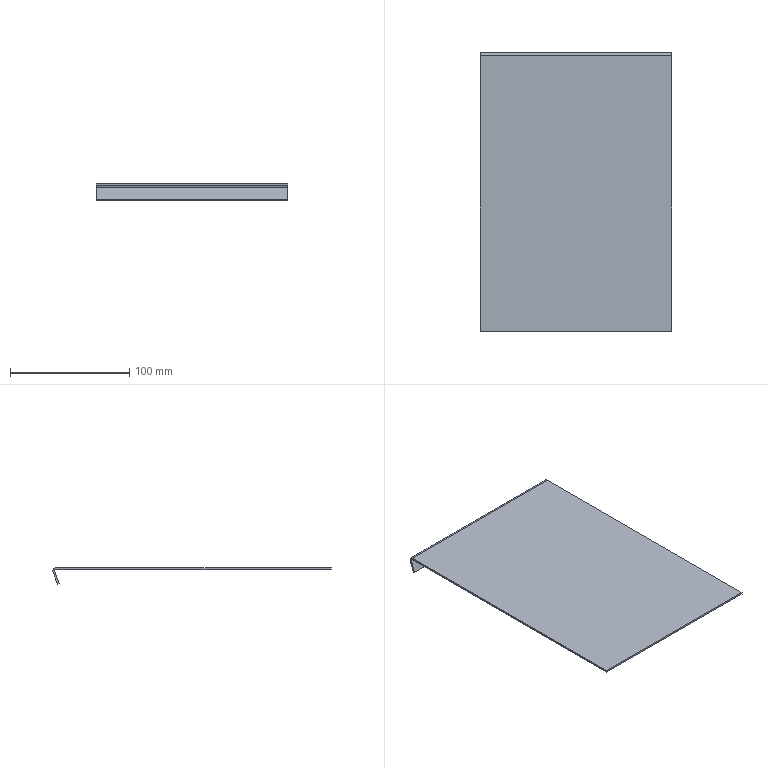Part | STEP file | 1-43.5 | 1 solid | 10 faces | box 160 x 233 x 13.692 mm | volume 58766 mm3 | plane 8 | cylinder 2 | commonest cylinder face diameters 2 x1 5 x1
STEP:
#1=CARTESIAN_POINT('',(0.,0.,0.));
#2=DIRECTION('',(0.,0.,1.));
#3=DIRECTION('',(1.,0.,0.));
#4=AXIS2_PLACEMENT_3D('',#1,#2,#3);
#5=CARTESIAN_POINT('',(-80.,0.,0.));
#6=VERTEX_POINT('',#5);
#7=CARTESIAN_POINT('',(-80.,0.,-1.5));
#8=VERTEX_POINT('',#7);
#9=CARTESIAN_POINT('',(-80.,0.,0.));
#10=DIRECTION('',(0.,0.,-1.));
#11=VECTOR('',#10,1.);
#12=LINE('',#9,#11);
#13=CARTESIAN_POINT('',(-80.,117.035,103.344));
#14=DIRECTION('',(1.,0.,0.));
#15=DIRECTION('',(0.,1.,0.));
#16=AXIS2_PLACEMENT_3D('',#13,#14,#15);
#17=PLANE('',#16);
#18=CARTESIAN_POINT('',(-117.035,-103.344));
#19=DIRECTION('',(0.,-1.));
#20=VECTOR('',#19,1.);
#21=LINE('',#18,#20);
#22=(GEOMETRIC_REPRESENTATION_CONTEXT(2)PARAMETRIC_REPRESENTATION_CONTEXT()REPRESENTATION_CONTEXT('',''));
#23=DEFINITIONAL_REPRESENTATION('',(#21),#22);
#24=PCURVE('',#17,#23);
#25=CARTESIAN_POINT('',(0.,0.,-0.75));
#26=DIRECTION('',(0.,-1.,0.));
#27=DIRECTION('',(0.,0.,-1.));
#28=AXIS2_PLACEMENT_3D('',#25,#26,#27);
#29=PLANE('',#28);
#30=CARTESIAN_POINT('',(-0.75,-80.));
#31=DIRECTION('',(1.,0.));
#32=VECTOR('',#31,1.);
#33=LINE('',#30,#32);
#34=(GEOMETRIC_REPRESENTATION_CONTEXT(2)PARAMETRIC_REPRESENTATION_CONTEXT()REPRESENTATION_CONTEXT('',''));
#35=DEFINITIONAL_REPRESENTATION('',(#33),#34);
#36=PCURVE('',#29,#35);
#37=SURFACE_CURVE('',#12,(#24,#36),.PCURVE_S1.);
#38=EDGE_CURVE('',#6,#8,#37,.T.);
#39=ORIENTED_EDGE('',*,*,#38,.T.);
#40=CARTESIAN_POINT('',(-80.,230.5,-1.5));
#41=VERTEX_POINT('',#40);
#42=CARTESIAN_POINT('',(-80.,0.,-1.5));
#43=DIRECTION('',(0.,1.,0.));
#44=VECTOR('',#43,1.);
#45=LINE('',#42,#44);
#46=CARTESIAN_POINT('',(-117.035,-104.844));
#47=DIRECTION('',(1.,0.));
#48=VECTOR('',#47,1.);
#49=LINE('',#46,#48);
#50=(GEOMETRIC_REPRESENTATION_CONTEXT(2)PARAMETRIC_REPRESENTATION_CONTEXT()REPRESENTATION_CONTEXT('',''));
#51=DEFINITIONAL_REPRESENTATION('',(#49),#50);
#52=PCURVE('',#17,#51);
#53=CARTESIAN_POINT('',(0.,115.25,-1.5));
#54=DIRECTION('',(0.,0.,-1.));
#55=DIRECTION('',(0.,1.,0.));
#56=AXIS2_PLACEMENT_3D('',#53,#54,#55);
#57=PLANE('',#56);
#58=CARTESIAN_POINT('',(-115.25,-80.));
#59=DIRECTION('',(1.,0.));
#60=VECTOR('',#59,1.);
#61=LINE('',#58,#60);
#62=(GEOMETRIC_REPRESENTATION_CONTEXT(2)PARAMETRIC_REPRESENTATION_CONTEXT()REPRESENTATION_CONTEXT('',''));
#63=DEFINITIONAL_REPRESENTATION('',(#61),#62);
#64=PCURVE('',#57,#63);
#65=SURFACE_CURVE('',#45,(#52,#64),.PCURVE_S1.);
#66=EDGE_CURVE('',#8,#41,#65,.T.);
#67=ORIENTED_EDGE('',*,*,#66,.T.);
#68=CARTESIAN_POINT('',(-80.,231.44,-2.842));
#69=VERTEX_POINT('',#68);
#70=CARTESIAN_POINT('',(-80.,230.5,-2.5));
#71=DIRECTION('',(-1.,0.,0.));
#72=DIRECTION('',(0.,0.,1.));
#73=AXIS2_PLACEMENT_3D('',#70,#71,#72);
#74=CIRCLE('',#73,1.);
#75=CARTESIAN_POINT('',(113.465,-104.844));
#76=CARTESIAN_POINT('',(115.197,-104.844));
#77=CARTESIAN_POINT('',(114.331,-106.344));
#78=CARTESIAN_POINT('',(113.465,-107.844));
#79=CARTESIAN_POINT('',(112.599,-106.344));
#80=CARTESIAN_POINT('',(111.733,-104.844));
#81=CARTESIAN_POINT('',(113.465,-104.844));
#82=(BOUNDED_CURVE()B_SPLINE_CURVE(2,(#75,#76,#77,#78,#79,#80,#81),.UNSPECIFIED.,.T.,.F.)B_SPLINE_CURVE_WITH_KNOTS((1,2,2,2,2,1),(-2.094,0.,2.094,4.189,6.283,8.378),.UNSPECIFIED.)CURVE()GEOMETRIC_REPRESENTATION_ITEM()RATIONAL_B_SPLINE_CURVE((1.,0.5,1.,0.5,1.,0.5,1.))REPRESENTATION_ITEM(''));
#83=(GEOMETRIC_REPRESENTATION_CONTEXT(2)PARAMETRIC_REPRESENTATION_CONTEXT()REPRESENTATION_CONTEXT('',''));
#84=DEFINITIONAL_REPRESENTATION('',(#82),#83);
#85=PCURVE('',#17,#84);
#86=CARTESIAN_POINT('',(-80.,230.5,-2.5));
#87=DIRECTION('',(1.,0.,0.));
#88=DIRECTION('',(0.,0.,1.));
#89=AXIS2_PLACEMENT_3D('',#86,#87,#88);
#90=CYLINDRICAL_SURFACE('',#89,1.);
#91=CARTESIAN_POINT('',(6.283,0.));
#92=DIRECTION('',(-1.,0.));
#93=VECTOR('',#92,1.);
#94=LINE('',#91,#93);
#95=(GEOMETRIC_REPRESENTATION_CONTEXT(2)PARAMETRIC_REPRESENTATION_CONTEXT()REPRESENTATION_CONTEXT('',''));
#96=DEFINITIONAL_REPRESENTATION('',(#94),#95);
#97=PCURVE('',#90,#96);
#98=SURFACE_CURVE('',#74,(#85,#97),.PCURVE_S1.);
#99=EDGE_CURVE('',#41,#69,#98,.T.);
#100=ORIENTED_EDGE('',*,*,#99,.T.);
#101=CARTESIAN_POINT('',(-80.,227.677,-13.179));
#102=VERTEX_POINT('',#101);
#103=CARTESIAN_POINT('',(-80.,231.44,-2.842));
#104=DIRECTION('',(0.,-0.342,-0.9397));
#105=VECTOR('',#104,1.);
#106=LINE('',#103,#105);
#107=CARTESIAN_POINT('',(114.405,-106.186));
#108=DIRECTION('',(-0.342,-0.9397));
#109=VECTOR('',#108,1.);
#110=LINE('',#107,#109);
#111=(GEOMETRIC_REPRESENTATION_CONTEXT(2)PARAMETRIC_REPRESENTATION_CONTEXT()REPRESENTATION_CONTEXT('',''));
#112=DEFINITIONAL_REPRESENTATION('',(#110),#111);
#113=PCURVE('',#17,#112);
#114=CARTESIAN_POINT('',(0.,229.559,-8.01));
#115=DIRECTION('',(0.,-0.9397,0.342));
#116=DIRECTION('',(0.,-0.342,-0.9397));
#117=AXIS2_PLACEMENT_3D('',#114,#115,#116);
#118=PLANE('',#117);
#119=CARTESIAN_POINT('',(-5.5,-80.));
#120=DIRECTION('',(1.,0.));
#121=VECTOR('',#120,1.);
#122=LINE('',#119,#121);
#123=(GEOMETRIC_REPRESENTATION_CONTEXT(2)PARAMETRIC_REPRESENTATION_CONTEXT()REPRESENTATION_CONTEXT('',''));
#124=DEFINITIONAL_REPRESENTATION('',(#122),#123);
#125=PCURVE('',#118,#124);
#126=SURFACE_CURVE('',#106,(#113,#125),.PCURVE_S1.);
#127=EDGE_CURVE('',#69,#102,#126,.T.);
#128=ORIENTED_EDGE('',*,*,#127,.T.);
#129=CARTESIAN_POINT('',(-80.,229.087,-13.692));
#130=VERTEX_POINT('',#129);
#131=CARTESIAN_POINT('',(-80.,227.677,-13.179));
#132=DIRECTION('',(0.,0.9397,-0.342));
#133=VECTOR('',#132,1.);
#134=LINE('',#131,#133);
#135=CARTESIAN_POINT('',(110.642,-116.522));
#136=DIRECTION('',(0.9397,-0.342));
#137=VECTOR('',#136,1.);
#138=LINE('',#135,#137);
#139=(GEOMETRIC_REPRESENTATION_CONTEXT(2)PARAMETRIC_REPRESENTATION_CONTEXT()REPRESENTATION_CONTEXT('',''));
#140=DEFINITIONAL_REPRESENTATION('',(#138),#139);
#141=PCURVE('',#17,#140);
#142=CARTESIAN_POINT('',(0.,228.382,-13.435));
#143=DIRECTION('',(0.,-0.342,-0.9397));
#144=DIRECTION('',(0.,0.9397,-0.342));
#145=AXIS2_PLACEMENT_3D('',#142,#143,#144);
#146=PLANE('',#145);
#147=CARTESIAN_POINT('',(-0.75,-80.));
#148=DIRECTION('',(1.,0.));
#149=VECTOR('',#148,1.);
#150=LINE('',#147,#149);
#151=(GEOMETRIC_REPRESENTATION_CONTEXT(2)PARAMETRIC_REPRESENTATION_CONTEXT()REPRESENTATION_CONTEXT('',''));
#152=DEFINITIONAL_REPRESENTATION('',(#150),#151);
#153=PCURVE('',#146,#152);
#154=SURFACE_CURVE('',#134,(#141,#153),.PCURVE_S1.);
#155=EDGE_CURVE('',#102,#130,#154,.T.);
#156=ORIENTED_EDGE('',*,*,#155,.T.);
#157=CARTESIAN_POINT('',(-80.,232.849,-3.355));
#158=VERTEX_POINT('',#157);
#159=CARTESIAN_POINT('',(-80.,229.087,-13.692));
#160=DIRECTION('',(0.,0.342,0.9397));
#161=VECTOR('',#160,1.);
#162=LINE('',#159,#161);
#163=CARTESIAN_POINT('',(112.052,-117.035));
#164=DIRECTION('',(0.342,0.9397));
#165=VECTOR('',#164,1.);
#166=LINE('',#163,#165);
#167=(GEOMETRIC_REPRESENTATION_CONTEXT(2)PARAMETRIC_REPRESENTATION_CONTEXT()REPRESENTATION_CONTEXT('',''));
#168=DEFINITIONAL_REPRESENTATION('',(#166),#167);
#169=PCURVE('',#17,#168);
#170=CARTESIAN_POINT('',(0.,230.968,-8.523));
#171=DIRECTION('',(0.,0.9397,-0.342));
#172=DIRECTION('',(0.,0.342,0.9397));
#173=AXIS2_PLACEMENT_3D('',#170,#171,#172);
#174=PLANE('',#173);
#175=CARTESIAN_POINT('',(-5.5,-80.));
#176=DIRECTION('',(1.,0.));
#177=VECTOR('',#176,1.);
#178=LINE('',#175,#177);
#179=(GEOMETRIC_REPRESENTATION_CONTEXT(2)PARAMETRIC_REPRESENTATION_CONTEXT()REPRESENTATION_CONTEXT('',''));
#180=DEFINITIONAL_REPRESENTATION('',(#178),#179);
#181=PCURVE('',#174,#180);
#182=SURFACE_CURVE('',#162,(#169,#181),.PCURVE_S1.);
#183=EDGE_CURVE('',#130,#158,#182,.T.);
#184=ORIENTED_EDGE('',*,*,#183,.T.);
#185=CARTESIAN_POINT('',(-80.,230.5,0.));
#186=VERTEX_POINT('',#185);
#187=CARTESIAN_POINT('',(-80.,230.5,-2.5));
#188=DIRECTION('',(1.,0.,0.));
#189=DIRECTION('',(0.,0.9397,-0.342));
#190=AXIS2_PLACEMENT_3D('',#187,#188,#189);
#191=CIRCLE('',#190,2.5);
#192=CARTESIAN_POINT('',(113.465,-105.844));
#193=DIRECTION('',(0.9397,-0.342));
#194=AXIS2_PLACEMENT_2D('',#192,#193);
#195=CIRCLE('',#194,2.5);
#196=(GEOMETRIC_REPRESENTATION_CONTEXT(2)PARAMETRIC_REPRESENTATION_CONTEXT()REPRESENTATION_CONTEXT('',''));
#197=DEFINITIONAL_REPRESENTATION('',(#195),#196);
#198=PCURVE('',#17,#197);
#199=CARTESIAN_POINT('',(-80.,230.5,-2.5));
#200=DIRECTION('',(1.,0.,0.));
#201=DIRECTION('',(0.,0.9397,-0.342));
#202=AXIS2_PLACEMENT_3D('',#199,#200,#201);
#203=CYLINDRICAL_SURFACE('',#202,2.5);
#204=CARTESIAN_POINT('',(0.,0.));
#205=DIRECTION('',(1.,0.));
#206=VECTOR('',#205,1.);
#207=LINE('',#204,#206);
#208=(GEOMETRIC_REPRESENTATION_CONTEXT(2)PARAMETRIC_REPRESENTATION_CONTEXT()REPRESENTATION_CONTEXT('',''));
#209=DEFINITIONAL_REPRESENTATION('',(#207),#208);
#210=PCURVE('',#203,#209);
#211=SURFACE_CURVE('',#191,(#198,#210),.PCURVE_S1.);
#212=EDGE_CURVE('',#158,#186,#211,.T.);
#213=ORIENTED_EDGE('',*,*,#212,.T.);
#214=CARTESIAN_POINT('',(-80.,230.5,0.));
#215=DIRECTION('',(0.,-1.,0.));
#216=VECTOR('',#215,1.);
#217=LINE('',#214,#216);
#218=CARTESIAN_POINT('',(113.465,-103.344));
#219=DIRECTION('',(-1.,0.));
#220=VECTOR('',#219,1.);
#221=LINE('',#218,#220);
#222=(GEOMETRIC_REPRESENTATION_CONTEXT(2)PARAMETRIC_REPRESENTATION_CONTEXT()REPRESENTATION_CONTEXT('',''));
#223=DEFINITIONAL_REPRESENTATION('',(#221),#222);
#224=PCURVE('',#17,#223);
#225=CARTESIAN_POINT('',(0.,115.25,0.));
#226=DIRECTION('',(0.,0.,1.));
#227=DIRECTION('',(0.,-1.,0.));
#228=AXIS2_PLACEMENT_3D('',#225,#226,#227);
#229=PLANE('',#228);
#230=CARTESIAN_POINT('',(-115.25,-80.));
#231=DIRECTION('',(1.,0.));
#232=VECTOR('',#231,1.);
#233=LINE('',#230,#232);
#234=(GEOMETRIC_REPRESENTATION_CONTEXT(2)PARAMETRIC_REPRESENTATION_CONTEXT()REPRESENTATION_CONTEXT('',''));
#235=DEFINITIONAL_REPRESENTATION('',(#233),#234);
#236=PCURVE('',#229,#235);
#237=SURFACE_CURVE('',#217,(#224,#236),.PCURVE_S1.);
#238=EDGE_CURVE('',#186,#6,#237,.T.);
#239=ORIENTED_EDGE('',*,*,#238,.T.);
#240=EDGE_LOOP('',(#39,#67,#100,#128,#156,#184,#213,#239));
#241=FACE_BOUND('',#240,.F.);
#242=ADVANCED_FACE('',(#241),#17,.F.);
#243=CARTESIAN_POINT('',(80.,0.,0.));
#244=VERTEX_POINT('',#243);
#245=CARTESIAN_POINT('',(80.,0.,-1.5));
#246=VERTEX_POINT('',#245);
#247=CARTESIAN_POINT('',(80.,0.,0.));
#248=DIRECTION('',(0.,0.,-1.));
#249=VECTOR('',#248,1.);
#250=LINE('',#247,#249);
#251=CARTESIAN_POINT('',(80.,117.035,103.344));
#252=DIRECTION('',(1.,0.,0.));
#253=DIRECTION('',(0.,1.,0.));
#254=AXIS2_PLACEMENT_3D('',#251,#252,#253);
#255=PLANE('',#254);
#256=CARTESIAN_POINT('',(-117.035,-103.344));
#257=DIRECTION('',(0.,-1.));
#258=VECTOR('',#257,1.);
#259=LINE('',#256,#258);
#260=(GEOMETRIC_REPRESENTATION_CONTEXT(2)PARAMETRIC_REPRESENTATION_CONTEXT()REPRESENTATION_CONTEXT('',''));
#261=DEFINITIONAL_REPRESENTATION('',(#259),#260);
#262=PCURVE('',#255,#261);
#263=CARTESIAN_POINT('',(-0.75,80.));
#264=DIRECTION('',(1.,0.));
#265=VECTOR('',#264,1.);
#266=LINE('',#263,#265);
#267=(GEOMETRIC_REPRESENTATION_CONTEXT(2)PARAMETRIC_REPRESENTATION_CONTEXT()REPRESENTATION_CONTEXT('',''));
#268=DEFINITIONAL_REPRESENTATION('',(#266),#267);
#269=PCURVE('',#29,#268);
#270=SURFACE_CURVE('',#250,(#262,#269),.PCURVE_S1.);
#271=EDGE_CURVE('',#244,#246,#270,.T.);
#272=ORIENTED_EDGE('',*,*,#271,.T.);
#273=CARTESIAN_POINT('',(80.,230.5,-1.5));
#274=VERTEX_POINT('',#273);
#275=CARTESIAN_POINT('',(80.,0.,-1.5));
#276=DIRECTION('',(0.,1.,0.));
#277=VECTOR('',#276,1.);
#278=LINE('',#275,#277);
#279=CARTESIAN_POINT('',(-117.035,-104.844));
#280=DIRECTION('',(1.,0.));
#281=VECTOR('',#280,1.);
#282=LINE('',#279,#281);
#283=(GEOMETRIC_REPRESENTATION_CONTEXT(2)PARAMETRIC_REPRESENTATION_CONTEXT()REPRESENTATION_CONTEXT('',''));
#284=DEFINITIONAL_REPRESENTATION('',(#282),#283);
#285=PCURVE('',#255,#284);
#286=CARTESIAN_POINT('',(-115.25,80.));
#287=DIRECTION('',(1.,0.));
#288=VECTOR('',#287,1.);
#289=LINE('',#286,#288);
#290=(GEOMETRIC_REPRESENTATION_CONTEXT(2)PARAMETRIC_REPRESENTATION_CONTEXT()REPRESENTATION_CONTEXT('',''));
#291=DEFINITIONAL_REPRESENTATION('',(#289),#290);
#292=PCURVE('',#57,#291);
#293=SURFACE_CURVE('',#278,(#285,#292),.PCURVE_S1.);
#294=EDGE_CURVE('',#246,#274,#293,.T.);
#295=ORIENTED_EDGE('',*,*,#294,.T.);
#296=CARTESIAN_POINT('',(80.,231.44,-2.842));
#297=VERTEX_POINT('',#296);
#298=CARTESIAN_POINT('',(80.,230.5,-2.5));
#299=DIRECTION('',(-1.,0.,0.));
#300=DIRECTION('',(0.,0.,1.));
#301=AXIS2_PLACEMENT_3D('',#298,#299,#300);
#302=CIRCLE('',#301,1.);
#303=CARTESIAN_POINT('',(113.465,-104.844));
#304=CARTESIAN_POINT('',(115.197,-104.844));
#305=CARTESIAN_POINT('',(114.331,-106.344));
#306=CARTESIAN_POINT('',(113.465,-107.844));
#307=CARTESIAN_POINT('',(112.599,-106.344));
#308=CARTESIAN_POINT('',(111.733,-104.844));
#309=CARTESIAN_POINT('',(113.465,-104.844));
#310=(BOUNDED_CURVE()B_SPLINE_CURVE(2,(#303,#304,#305,#306,#307,#308,#309),.UNSPECIFIED.,.T.,.F.)B_SPLINE_CURVE_WITH_KNOTS((1,2,2,2,2,1),(-2.094,0.,2.094,4.189,6.283,8.378),.UNSPECIFIED.)CURVE()GEOMETRIC_REPRESENTATION_ITEM()RATIONAL_B_SPLINE_CURVE((1.,0.5,1.,0.5,1.,0.5,1.))REPRESENTATION_ITEM(''));
#311=(GEOMETRIC_REPRESENTATION_CONTEXT(2)PARAMETRIC_REPRESENTATION_CONTEXT()REPRESENTATION_CONTEXT('',''));
#312=DEFINITIONAL_REPRESENTATION('',(#310),#311);
#313=PCURVE('',#255,#312);
#314=CARTESIAN_POINT('',(6.283,160.));
#315=DIRECTION('',(-1.,0.));
#316=VECTOR('',#315,1.);
#317=LINE('',#314,#316);
#318=(GEOMETRIC_REPRESENTATION_CONTEXT(2)PARAMETRIC_REPRESENTATION_CONTEXT()REPRESENTATION_CONTEXT('',''));
#319=DEFINITIONAL_REPRESENTATION('',(#317),#318);
#320=PCURVE('',#90,#319);
#321=SURFACE_CURVE('',#302,(#313,#320),.PCURVE_S1.);
#322=EDGE_CURVE('',#274,#297,#321,.T.);
#323=ORIENTED_EDGE('',*,*,#322,.T.);
#324=CARTESIAN_POINT('',(80.,227.677,-13.179));
#325=VERTEX_POINT('',#324);
#326=CARTESIAN_POINT('',(80.,231.44,-2.842));
#327=DIRECTION('',(0.,-0.342,-0.9397));
#328=VECTOR('',#327,1.);
#329=LINE('',#326,#328);
#330=CARTESIAN_POINT('',(114.405,-106.186));
#331=DIRECTION('',(-0.342,-0.9397));
#332=VECTOR('',#331,1.);
#333=LINE('',#330,#332);
#334=(GEOMETRIC_REPRESENTATION_CONTEXT(2)PARAMETRIC_REPRESENTATION_CONTEXT()REPRESENTATION_CONTEXT('',''));
#335=DEFINITIONAL_REPRESENTATION('',(#333),#334);
#336=PCURVE('',#255,#335);
#337=CARTESIAN_POINT('',(-5.5,80.));
#338=DIRECTION('',(1.,0.));
#339=VECTOR('',#338,1.);
#340=LINE('',#337,#339);
#341=(GEOMETRIC_REPRESENTATION_CONTEXT(2)PARAMETRIC_REPRESENTATION_CONTEXT()REPRESENTATION_CONTEXT('',''));
#342=DEFINITIONAL_REPRESENTATION('',(#340),#341);
#343=PCURVE('',#118,#342);
#344=SURFACE_CURVE('',#329,(#336,#343),.PCURVE_S1.);
#345=EDGE_CURVE('',#297,#325,#344,.T.);
#346=ORIENTED_EDGE('',*,*,#345,.T.);
#347=CARTESIAN_POINT('',(80.,229.087,-13.692));
#348=VERTEX_POINT('',#347);
#349=CARTESIAN_POINT('',(80.,227.677,-13.179));
#350=DIRECTION('',(0.,0.9397,-0.342));
#351=VECTOR('',#350,1.);
#352=LINE('',#349,#351);
#353=CARTESIAN_POINT('',(110.642,-116.522));
#354=DIRECTION('',(0.9397,-0.342));
#355=VECTOR('',#354,1.);
#356=LINE('',#353,#355);
#357=(GEOMETRIC_REPRESENTATION_CONTEXT(2)PARAMETRIC_REPRESENTATION_CONTEXT()REPRESENTATION_CONTEXT('',''));
#358=DEFINITIONAL_REPRESENTATION('',(#356),#357);
#359=PCURVE('',#255,#358);
#360=CARTESIAN_POINT('',(-0.75,80.));
#361=DIRECTION('',(1.,0.));
#362=VECTOR('',#361,1.);
#363=LINE('',#360,#362);
#364=(GEOMETRIC_REPRESENTATION_CONTEXT(2)PARAMETRIC_REPRESENTATION_CONTEXT()REPRESENTATION_CONTEXT('',''));
#365=DEFINITIONAL_REPRESENTATION('',(#363),#364);
#366=PCURVE('',#146,#365);
#367=SURFACE_CURVE('',#352,(#359,#366),.PCURVE_S1.);
#368=EDGE_CURVE('',#325,#348,#367,.T.);
#369=ORIENTED_EDGE('',*,*,#368,.T.);
#370=CARTESIAN_POINT('',(80.,232.849,-3.355));
#371=VERTEX_POINT('',#370);
#372=CARTESIAN_POINT('',(80.,229.087,-13.692));
#373=DIRECTION('',(0.,0.342,0.9397));
#374=VECTOR('',#373,1.);
#375=LINE('',#372,#374);
#376=CARTESIAN_POINT('',(112.052,-117.035));
#377=DIRECTION('',(0.342,0.9397));
#378=VECTOR('',#377,1.);
#379=LINE('',#376,#378);
#380=(GEOMETRIC_REPRESENTATION_CONTEXT(2)PARAMETRIC_REPRESENTATION_CONTEXT()REPRESENTATION_CONTEXT('',''));
#381=DEFINITIONAL_REPRESENTATION('',(#379),#380);
#382=PCURVE('',#255,#381);
#383=CARTESIAN_POINT('',(-5.5,80.));
#384=DIRECTION('',(1.,0.));
#385=VECTOR('',#384,1.);
#386=LINE('',#383,#385);
#387=(GEOMETRIC_REPRESENTATION_CONTEXT(2)PARAMETRIC_REPRESENTATION_CONTEXT()REPRESENTATION_CONTEXT('',''));
#388=DEFINITIONAL_REPRESENTATION('',(#386),#387);
#389=PCURVE('',#174,#388);
#390=SURFACE_CURVE('',#375,(#382,#389),.PCURVE_S1.);
#391=EDGE_CURVE('',#348,#371,#390,.T.);
#392=ORIENTED_EDGE('',*,*,#391,.T.);
#393=CARTESIAN_POINT('',(80.,230.5,0.));
#394=VERTEX_POINT('',#393);
#395=CARTESIAN_POINT('',(80.,230.5,-2.5));
#396=DIRECTION('',(1.,0.,0.));
#397=DIRECTION('',(0.,0.9397,-0.342));
#398=AXIS2_PLACEMENT_3D('',#395,#396,#397);
#399=CIRCLE('',#398,2.5);
#400=CARTESIAN_POINT('',(113.465,-105.844));
#401=DIRECTION('',(0.9397,-0.342));
#402=AXIS2_PLACEMENT_2D('',#400,#401);
#403=CIRCLE('',#402,2.5);
#404=(GEOMETRIC_REPRESENTATION_CONTEXT(2)PARAMETRIC_REPRESENTATION_CONTEXT()REPRESENTATION_CONTEXT('',''));
#405=DEFINITIONAL_REPRESENTATION('',(#403),#404);
#406=PCURVE('',#255,#405);
#407=CARTESIAN_POINT('',(0.,160.));
#408=DIRECTION('',(1.,0.));
#409=VECTOR('',#408,1.);
#410=LINE('',#407,#409);
#411=(GEOMETRIC_REPRESENTATION_CONTEXT(2)PARAMETRIC_REPRESENTATION_CONTEXT()REPRESENTATION_CONTEXT('',''));
#412=DEFINITIONAL_REPRESENTATION('',(#410),#411);
#413=PCURVE('',#203,#412);
#414=SURFACE_CURVE('',#399,(#406,#413),.PCURVE_S1.);
#415=EDGE_CURVE('',#371,#394,#414,.T.);
#416=ORIENTED_EDGE('',*,*,#415,.T.);
#417=CARTESIAN_POINT('',(80.,230.5,0.));
#418=DIRECTION('',(0.,-1.,0.));
#419=VECTOR('',#418,1.);
#420=LINE('',#417,#419);
#421=CARTESIAN_POINT('',(113.465,-103.344));
#422=DIRECTION('',(-1.,0.));
#423=VECTOR('',#422,1.);
#424=LINE('',#421,#423);
#425=(GEOMETRIC_REPRESENTATION_CONTEXT(2)PARAMETRIC_REPRESENTATION_CONTEXT()REPRESENTATION_CONTEXT('',''));
#426=DEFINITIONAL_REPRESENTATION('',(#424),#425);
#427=PCURVE('',#255,#426);
#428=CARTESIAN_POINT('',(-115.25,80.));
#429=DIRECTION('',(1.,0.));
#430=VECTOR('',#429,1.);
#431=LINE('',#428,#430);
#432=(GEOMETRIC_REPRESENTATION_CONTEXT(2)PARAMETRIC_REPRESENTATION_CONTEXT()REPRESENTATION_CONTEXT('',''));
#433=DEFINITIONAL_REPRESENTATION('',(#431),#432);
#434=PCURVE('',#229,#433);
#435=SURFACE_CURVE('',#420,(#427,#434),.PCURVE_S1.);
#436=EDGE_CURVE('',#394,#244,#435,.T.);
#437=ORIENTED_EDGE('',*,*,#436,.T.);
#438=EDGE_LOOP('',(#272,#295,#323,#346,#369,#392,#416,#437));
#439=FACE_BOUND('',#438,.T.);
#440=ADVANCED_FACE('',(#439),#255,.T.);
#441=ORIENTED_EDGE('',*,*,#38,.T.);
#442=CARTESIAN_POINT('',(-80.,0.,-1.5));
#443=DIRECTION('',(1.,0.,0.));
#444=VECTOR('',#443,1.);
#445=LINE('',#442,#444);
#446=CARTESIAN_POINT('',(0.75,-80.));
#447=DIRECTION('',(0.,1.));
#448=VECTOR('',#447,1.);
#449=LINE('',#446,#448);
#450=(GEOMETRIC_REPRESENTATION_CONTEXT(2)PARAMETRIC_REPRESENTATION_CONTEXT()REPRESENTATION_CONTEXT('',''));
#451=DEFINITIONAL_REPRESENTATION('',(#449),#450);
#452=PCURVE('',#29,#451);
#453=CARTESIAN_POINT('',(-115.25,-80.));
#454=DIRECTION('',(0.,1.));
#455=VECTOR('',#454,1.);
#456=LINE('',#453,#455);
#457=(GEOMETRIC_REPRESENTATION_CONTEXT(2)PARAMETRIC_REPRESENTATION_CONTEXT()REPRESENTATION_CONTEXT('',''));
#458=DEFINITIONAL_REPRESENTATION('',(#456),#457);
#459=PCURVE('',#57,#458);
#460=SURFACE_CURVE('',#445,(#452,#459),.PCURVE_S1.);
#461=EDGE_CURVE('',#8,#246,#460,.T.);
#462=ORIENTED_EDGE('',*,*,#461,.T.);
#463=ORIENTED_EDGE('',*,*,#271,.F.);
#464=CARTESIAN_POINT('',(-80.,0.,0.));
#465=DIRECTION('',(1.,0.,0.));
#466=VECTOR('',#465,1.);
#467=LINE('',#464,#466);
#468=CARTESIAN_POINT('',(-0.75,-80.));
#469=DIRECTION('',(0.,1.));
#470=VECTOR('',#469,1.);
#471=LINE('',#468,#470);
#472=(GEOMETRIC_REPRESENTATION_CONTEXT(2)PARAMETRIC_REPRESENTATION_CONTEXT()REPRESENTATION_CONTEXT('',''));
#473=DEFINITIONAL_REPRESENTATION('',(#471),#472);
#474=PCURVE('',#29,#473);
#475=CARTESIAN_POINT('',(115.25,-80.));
#476=DIRECTION('',(0.,1.));
#477=VECTOR('',#476,1.);
#478=LINE('',#475,#477);
#479=(GEOMETRIC_REPRESENTATION_CONTEXT(2)PARAMETRIC_REPRESENTATION_CONTEXT()REPRESENTATION_CONTEXT('',''));
#480=DEFINITIONAL_REPRESENTATION('',(#478),#479);
#481=PCURVE('',#229,#480);
#482=SURFACE_CURVE('',#467,(#474,#481),.PCURVE_S1.);
#483=EDGE_CURVE('',#6,#244,#482,.T.);
#484=ORIENTED_EDGE('',*,*,#483,.F.);
#485=EDGE_LOOP('',(#441,#462,#463,#484));
#486=FACE_BOUND('',#485,.T.);
#487=ADVANCED_FACE('',(#486),#29,.T.);
#488=ORIENTED_EDGE('',*,*,#66,.T.);
#489=CARTESIAN_POINT('',(-80.,230.5,-1.5));
#490=DIRECTION('',(1.,0.,0.));
#491=VECTOR('',#490,1.);
#492=LINE('',#489,#491);
#493=CARTESIAN_POINT('',(115.25,-80.));
#494=DIRECTION('',(0.,1.));
#495=VECTOR('',#494,1.);
#496=LINE('',#493,#495);
#497=(GEOMETRIC_REPRESENTATION_CONTEXT(2)PARAMETRIC_REPRESENTATION_CONTEXT()REPRESENTATION_CONTEXT('',''));
#498=DEFINITIONAL_REPRESENTATION('',(#496),#497);
#499=PCURVE('',#57,#498);
#500=CARTESIAN_POINT('',(6.283,0.));
#501=DIRECTION('',(0.,1.));
#502=VECTOR('',#501,1.);
#503=LINE('',#500,#502);
#504=(GEOMETRIC_REPRESENTATION_CONTEXT(2)PARAMETRIC_REPRESENTATION_CONTEXT()REPRESENTATION_CONTEXT('',''));
#505=DEFINITIONAL_REPRESENTATION('',(#503),#504);
#506=PCURVE('',#90,#505);
#507=SURFACE_CURVE('',#492,(#499,#506),.PCURVE_S1.);
#508=EDGE_CURVE('',#41,#274,#507,.T.);
#509=ORIENTED_EDGE('',*,*,#508,.T.);
#510=ORIENTED_EDGE('',*,*,#294,.F.);
#511=ORIENTED_EDGE('',*,*,#461,.F.);
#512=EDGE_LOOP('',(#488,#509,#510,#511));
#513=FACE_BOUND('',#512,.T.);
#514=ADVANCED_FACE('',(#513),#57,.T.);
#515=ORIENTED_EDGE('',*,*,#508,.T.);
#516=ORIENTED_EDGE('',*,*,#322,.T.);
#517=CARTESIAN_POINT('',(-80.,231.44,-2.842));
#518=DIRECTION('',(1.,0.,0.));
#519=VECTOR('',#518,1.);
#520=LINE('',#517,#519);
#521=CARTESIAN_POINT('',(4.363,0.));
#522=DIRECTION('',(0.,1.));
#523=VECTOR('',#522,1.);
#524=LINE('',#521,#523);
#525=(GEOMETRIC_REPRESENTATION_CONTEXT(2)PARAMETRIC_REPRESENTATION_CONTEXT()REPRESENTATION_CONTEXT('',''));
#526=DEFINITIONAL_REPRESENTATION('',(#524),#525);
#527=PCURVE('',#90,#526);
#528=CARTESIAN_POINT('',(-5.5,-80.));
#529=DIRECTION('',(0.,1.));
#530=VECTOR('',#529,1.);
#531=LINE('',#528,#530);
#532=(GEOMETRIC_REPRESENTATION_CONTEXT(2)PARAMETRIC_REPRESENTATION_CONTEXT()REPRESENTATION_CONTEXT('',''));
#533=DEFINITIONAL_REPRESENTATION('',(#531),#532);
#534=PCURVE('',#118,#533);
#535=SURFACE_CURVE('',#520,(#527,#534),.PCURVE_S1.);
#536=EDGE_CURVE('',#69,#297,#535,.T.);
#537=ORIENTED_EDGE('',*,*,#536,.F.);
#538=ORIENTED_EDGE('',*,*,#99,.F.);
#539=EDGE_LOOP('',(#515,#516,#537,#538));
#540=FACE_BOUND('',#539,.F.);
#541=ADVANCED_FACE('',(#540),#90,.F.);
#542=ORIENTED_EDGE('',*,*,#127,.T.);
#543=CARTESIAN_POINT('',(-80.,227.677,-13.179));
#544=DIRECTION('',(1.,0.,0.));
#545=VECTOR('',#544,1.);
#546=LINE('',#543,#545);
#547=CARTESIAN_POINT('',(5.5,-80.));
#548=DIRECTION('',(0.,1.));
#549=VECTOR('',#548,1.);
#550=LINE('',#547,#549);
#551=(GEOMETRIC_REPRESENTATION_CONTEXT(2)PARAMETRIC_REPRESENTATION_CONTEXT()REPRESENTATION_CONTEXT('',''));
#552=DEFINITIONAL_REPRESENTATION('',(#550),#551);
#553=PCURVE('',#118,#552);
#554=CARTESIAN_POINT('',(-0.75,-80.));
#555=DIRECTION('',(0.,1.));
#556=VECTOR('',#555,1.);
#557=LINE('',#554,#556);
#558=(GEOMETRIC_REPRESENTATION_CONTEXT(2)PARAMETRIC_REPRESENTATION_CONTEXT()REPRESENTATION_CONTEXT('',''));
#559=DEFINITIONAL_REPRESENTATION('',(#557),#558);
#560=PCURVE('',#146,#559);
#561=SURFACE_CURVE('',#546,(#553,#560),.PCURVE_S1.);
#562=EDGE_CURVE('',#102,#325,#561,.T.);
#563=ORIENTED_EDGE('',*,*,#562,.T.);
#564=ORIENTED_EDGE('',*,*,#345,.F.);
#565=ORIENTED_EDGE('',*,*,#536,.F.);
#566=EDGE_LOOP('',(#542,#563,#564,#565));
#567=FACE_BOUND('',#566,.T.);
#568=ADVANCED_FACE('',(#567),#118,.T.);
#569=ORIENTED_EDGE('',*,*,#155,.T.);
#570=CARTESIAN_POINT('',(-80.,229.087,-13.692));
#571=DIRECTION('',(1.,0.,0.));
#572=VECTOR('',#571,1.);
#573=LINE('',#570,#572);
#574=CARTESIAN_POINT('',(0.75,-80.));
#575=DIRECTION('',(0.,1.));
#576=VECTOR('',#575,1.);
#577=LINE('',#574,#576);
#578=(GEOMETRIC_REPRESENTATION_CONTEXT(2)PARAMETRIC_REPRESENTATION_CONTEXT()REPRESENTATION_CONTEXT('',''));
#579=DEFINITIONAL_REPRESENTATION('',(#577),#578);
#580=PCURVE('',#146,#579);
#581=CARTESIAN_POINT('',(-5.5,-80.));
#582=DIRECTION('',(0.,1.));
#583=VECTOR('',#582,1.);
#584=LINE('',#581,#583);
#585=(GEOMETRIC_REPRESENTATION_CONTEXT(2)PARAMETRIC_REPRESENTATION_CONTEXT()REPRESENTATION_CONTEXT('',''));
#586=DEFINITIONAL_REPRESENTATION('',(#584),#585);
#587=PCURVE('',#174,#586);
#588=SURFACE_CURVE('',#573,(#580,#587),.PCURVE_S1.);
#589=EDGE_CURVE('',#130,#348,#588,.T.);
#590=ORIENTED_EDGE('',*,*,#589,.T.);
#591=ORIENTED_EDGE('',*,*,#368,.F.);
#592=ORIENTED_EDGE('',*,*,#562,.F.);
#593=EDGE_LOOP('',(#569,#590,#591,#592));
#594=FACE_BOUND('',#593,.T.);
#595=ADVANCED_FACE('',(#594),#146,.T.);
#596=ORIENTED_EDGE('',*,*,#183,.T.);
#597=CARTESIAN_POINT('',(-80.,232.849,-3.355));
#598=DIRECTION('',(1.,0.,0.));
#599=VECTOR('',#598,1.);
#600=LINE('',#597,#599);
#601=CARTESIAN_POINT('',(5.5,-80.));
#602=DIRECTION('',(0.,1.));
#603=VECTOR('',#602,1.);
#604=LINE('',#601,#603);
#605=(GEOMETRIC_REPRESENTATION_CONTEXT(2)PARAMETRIC_REPRESENTATION_CONTEXT()REPRESENTATION_CONTEXT('',''));
#606=DEFINITIONAL_REPRESENTATION('',(#604),#605);
#607=PCURVE('',#174,#606);
#608=CARTESIAN_POINT('',(0.,0.));
#609=DIRECTION('',(0.,1.));
#610=VECTOR('',#609,1.);
#611=LINE('',#608,#610);
#612=(GEOMETRIC_REPRESENTATION_CONTEXT(2)PARAMETRIC_REPRESENTATION_CONTEXT()REPRESENTATION_CONTEXT('',''));
#613=DEFINITIONAL_REPRESENTATION('',(#611),#612);
#614=PCURVE('',#203,#613);
#615=SURFACE_CURVE('',#600,(#607,#614),.PCURVE_S1.);
#616=EDGE_CURVE('',#158,#371,#615,.T.);
#617=ORIENTED_EDGE('',*,*,#616,.T.);
#618=ORIENTED_EDGE('',*,*,#391,.F.);
#619=ORIENTED_EDGE('',*,*,#589,.F.);
#620=EDGE_LOOP('',(#596,#617,#618,#619));
#621=FACE_BOUND('',#620,.T.);
#622=ADVANCED_FACE('',(#621),#174,.T.);
#623=ORIENTED_EDGE('',*,*,#212,.T.);
#624=CARTESIAN_POINT('',(-80.,230.5,0.));
#625=DIRECTION('',(1.,0.,0.));
#626=VECTOR('',#625,1.);
#627=LINE('',#624,#626);
#628=CARTESIAN_POINT('',(1.92,0.));
#629=DIRECTION('',(0.,1.));
#630=VECTOR('',#629,1.);
#631=LINE('',#628,#630);
#632=(GEOMETRIC_REPRESENTATION_CONTEXT(2)PARAMETRIC_REPRESENTATION_CONTEXT()REPRESENTATION_CONTEXT('',''));
#633=DEFINITIONAL_REPRESENTATION('',(#631),#632);
#634=PCURVE('',#203,#633);
#635=CARTESIAN_POINT('',(-115.25,-80.));
#636=DIRECTION('',(0.,1.));
#637=VECTOR('',#636,1.);
#638=LINE('',#635,#637);
#639=(GEOMETRIC_REPRESENTATION_CONTEXT(2)PARAMETRIC_REPRESENTATION_CONTEXT()REPRESENTATION_CONTEXT('',''));
#640=DEFINITIONAL_REPRESENTATION('',(#638),#639);
#641=PCURVE('',#229,#640);
#642=SURFACE_CURVE('',#627,(#634,#641),.PCURVE_S1.);
#643=EDGE_CURVE('',#186,#394,#642,.T.);
#644=ORIENTED_EDGE('',*,*,#643,.T.);
#645=ORIENTED_EDGE('',*,*,#415,.F.);
#646=ORIENTED_EDGE('',*,*,#616,.F.);
#647=EDGE_LOOP('',(#623,#644,#645,#646));
#648=FACE_BOUND('',#647,.T.);
#649=ADVANCED_FACE('',(#648),#203,.T.);
#650=ORIENTED_EDGE('',*,*,#238,.T.);
#651=ORIENTED_EDGE('',*,*,#483,.T.);
#652=ORIENTED_EDGE('',*,*,#436,.F.);
#653=ORIENTED_EDGE('',*,*,#643,.F.);
#654=EDGE_LOOP('',(#650,#651,#652,#653));
#655=FACE_BOUND('',#654,.T.);
#656=ADVANCED_FACE('',(#655),#229,.T.);
#657=CLOSED_SHELL('',(#242,#440,#487,#514,#541,#568,#595,#622,#649,#656));
#658=MANIFOLD_SOLID_BREP('',#657);
#659=(LENGTH_UNIT()NAMED_UNIT(*)SI_UNIT(.MILLI.,.METRE.));
#660=UNCERTAINTY_MEASURE_WITH_UNIT(LENGTH_MEASURE(0.0000001),#659,'','');
#661=(NAMED_UNIT(*)PLANE_ANGLE_UNIT()SI_UNIT($,.RADIAN.));
#662=(NAMED_UNIT(*)SI_UNIT($,.STERADIAN.)SOLID_ANGLE_UNIT());
#663=(GEOMETRIC_REPRESENTATION_CONTEXT(3)GLOBAL_UNCERTAINTY_ASSIGNED_CONTEXT((#660))GLOBAL_UNIT_ASSIGNED_CONTEXT((#659,#661,#662))REPRESENTATION_CONTEXT('',''));
#664=ADVANCED_BREP_SHAPE_REPRESENTATION('',(#4,#658),#663);